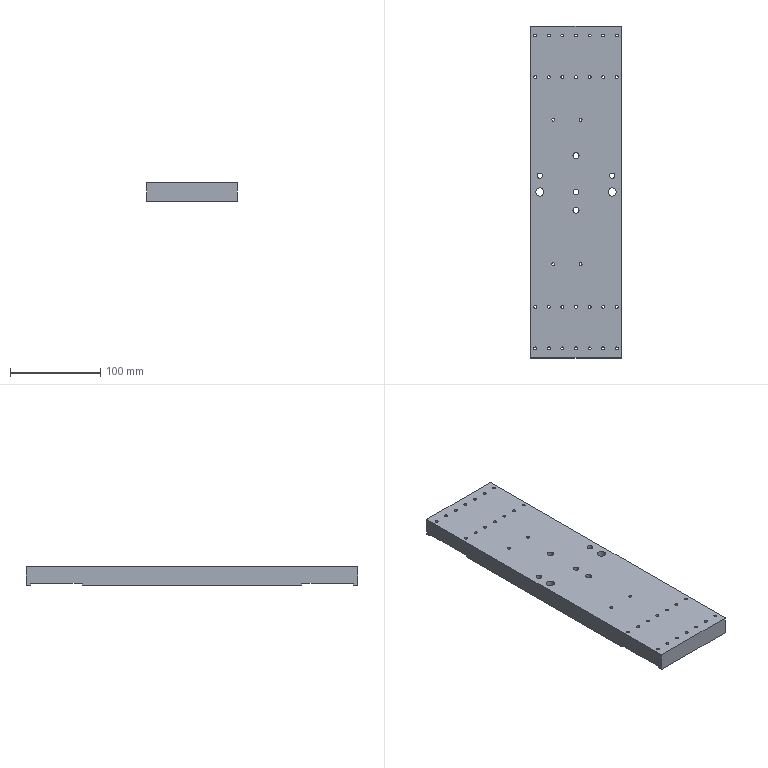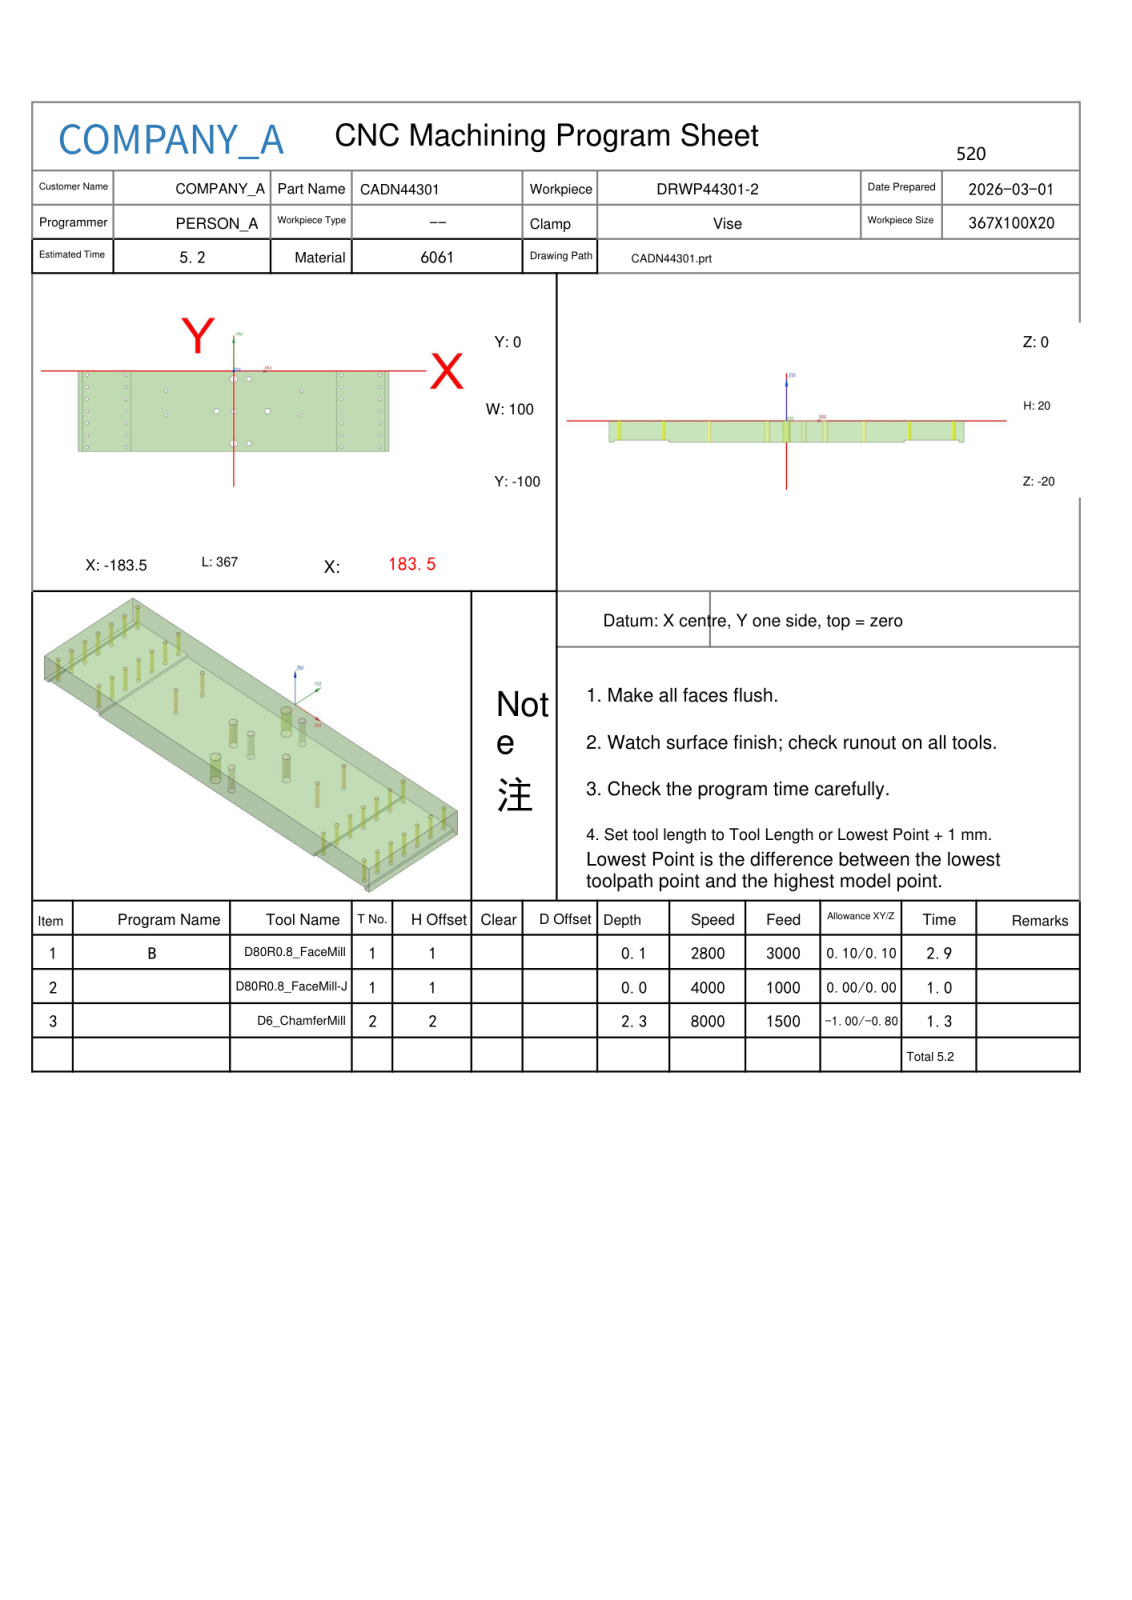NC program | NX | posted by the shop | part box 100 x 367 x 20 mm
Whole program:
%
O0001
(Machine time: 5.71 MIN)
(===Total Tool:2===)
(T1=D80R0.8 FaceMill D=80.  R=0.8  D-  H01 Z=-0.   )
(T2=D6_ChamferMill   D=6.   R=0.   D-  H02 Z=-2.3  )
G80 G90 G17 G49 G40
G91 G28 Z0
M01
N1 T01 M06
(D80R0.8 FaceMill  D=80. R=0.8 H=01 ce=0.10 di=0.10)
G00 G90 G54 X-235.597 Y-23.903 M03 S2800
G43 H01 Z50.
M08
Z6.011
G01 Z4.011 F3000.
X-223.597
X216.397
G02 X223.597 Y-31.103 I0.0 J-7.2
G01 Y-60.737
G02 X215.597 Y-68.737 I-8. J0.0
G01 X-223.597
X-235.597
Z6.011
G00 Y-23.903
Z5.522
G01 Z3.522
X-223.597
X216.397
G02 X223.597 Y-31.103 I0.0 J-7.2
G01 Y-60.737
G02 X215.597 Y-68.737 I-8. J0.0
G01 X-223.597
X-235.597
Z5.522
G00 Y-23.903
Z5.033
G01 Z3.033
X-223.597
X216.397
G02 X223.597 Y-31.103 I0.0 J-7.2
G01 Y-60.737
G02 X215.597 Y-68.737 I-8. J0.0
G01 X-223.597
X-235.597
Z5.033
G00 Y-23.903
Z4.544
G01 Z2.544
X-223.597
X216.397
G02 X223.597 Y-31.103 I0.0 J-7.2
G01 Y-60.737
G02 X215.597 Y-68.737 I-8. J0.0
G01 X-223.597
X-235.597
Z4.544
G00 Y-23.903
Z4.056
G01 Z2.056
X-223.597
X216.397
G02 X223.597 Y-31.103 I0.0 J-7.2
G01 Y-60.737
G02 X215.597 Y-68.737 I-8. J0.0
G01 X-223.597
X-235.597
Z4.056
G00 Y-23.903
Z3.567
G01 Z1.567
X-223.597
X216.397
G02 X223.597 Y-31.103 I0.0 J-7.2
G01 Y-60.737
G02 X215.597 Y-68.737 I-8. J0.0
G01 X-223.597
X-235.597
Z3.567
G00 Y-23.903
Z3.078
G01 Z1.078
X-223.597
X216.397
G02 X223.597 Y-31.103 I0.0 J-7.2
G01 Y-60.737
G02 X215.597 Y-68.737 I-8. J0.0
G01 X-223.597
X-235.597
Z3.078
G00 Y-23.903
Z2.589
G01 Z.589
X-223.597
X216.397
G02 X223.597 Y-31.103 I0.0 J-7.2
G01 Y-60.737
G02 X215.597 Y-68.737 I-8. J0.0
G01 X-223.597
X-235.597
Z2.589
G00 Y-23.903
Z2.1
G01 Z.1
X-223.597
X216.397
G02 X223.597 Y-31.103 I0.0 J-7.2
G01 Y-60.737
G02 X215.597 Y-68.737 I-8. J0.0
G01 X-223.597
X-235.597
Z2.1
G00 Z50.
G91 G28 Z0.0
M05
M09
G91 G28 Z0.0
M01
N2 T01 M06
(D80R0.8 FaceMill-J  D=80. R=0.8 H=01 ce=0.00 di=0.00)
G00 G90 G54 X-235.499 Y-24.001 M03 S4000
G43 H01 Z50.
M08
Z2.
G01 Z0.0 F1000.
X-223.499
X216.299
G02 X223.499 Y-31.201 I0.0 J-7.2
G01 Y-60.639
G02 X215.499 Y-68.639 I-8. J0.0
G01 X-223.499
X-235.499
Z2.
G00 Z50.
G91 G28 Z0.0
M05
M09
G91 G28 Z0.0
M01
N3 T02 M06
(D6_ChamferMill  D=6. R=0. H=02 ce=0.00 di=0.00)
G00 G90 G54 X-173. Y-95. M03 S8000
G43 H02 Z50.
M08
G98 G81 X-173. Y-95. Z-2.2 R3. F1000.
Y-80.
Y-65.
Y-50.
Y-35.
Y-20.
Y-5.
X-127.
Y-20.
Y-35.
Y-50.
Y-65.
Y-80.
Y-95.
X-80. Y-55.
Y-25.
X80. Y-55.
Y-25.
X127. Y-5.
Y-20.
Y-35.
Y-50.
Y-65.
Y-80.
Y-95.
X173.
Y-80.
Y-65.
Y-50.
Y-35.
Y-20.
Y-5.
G80
G00 Z50.
G00 G90 X17.13 Y-10.232 M03 S8000
Z50.
Z-.9
G01 Z-1.4 F600.
X16.5 Y-10.4
G03 X18. Y-11.9 I1.5 J0.0
X19.9 Y-10. I0.0 J1.9
X18. Y-8.1 I-1.9 J0.0
X16.1 Y-10. I0.0 J-1.9
X18. Y-11.9 I1.9 J0.0
X19.5 Y-10.4 I0.0 J1.5
G01 X18.87 Y-10.232
Z-.9
G00 Z50.
X-.87 Y-50.232
Z-.9
G01 Z-1.4
X-1.5 Y-50.4
G03 X0.0 Y-51.9 I1.5 J0.0
X1.9 Y-50. I0.0 J1.9
X0.0 Y-48.1 I-1.9 J0.0
X-1.9 Y-50. I0.0 J-1.9
X0.0 Y-51.9 I1.9 J0.0
X1.5 Y-50.4 I0.0 J1.5
G01 X.87 Y-50.232
Z-.9
G00 Z50.
X17.13 Y-90.232
Z-.9
G01 Z-1.4
X16.5 Y-90.4
G03 X18. Y-91.9 I1.5 J0.0
X19.9 Y-90. I0.0 J1.9
X18. Y-88.1 I-1.9 J0.0
X16.1 Y-90. I0.0 J-1.9
X18. Y-91.9 I1.9 J0.0
X19.5 Y-90.4 I0.0 J1.5
G01 X18.87 Y-90.232
Z-.9
G00 Z50.
G00 G90 X-22. Y-50. M03 S8000
Z50.
Z-.9
G01 Z-1.4 F600.
X-23.
G03 X-20. Y-53. I3. J0.0
X-17. Y-50. I0.0 J3.
X-20. Y-47. I-3. J0.0
X-23. Y-50. I0.0 J-3.
X-20. Y-53. I3. J0.0
X-17. Y-50. I0.0 J3.
G01 X-18.
Z-.9
G00 Z50.
X38.
Z-.9
G01 Z-1.4
X37.
G03 X40. Y-53. I3. J0.0
X43. Y-50. I0.0 J3.
X40. Y-47. I-3. J0.0
X37. Y-50. I0.0 J-3.
X40. Y-53. I3. J0.0
X43. Y-50. I0.0 J3.
G01 X42.
Z-.9
G00 Z50.
G00 G90 X1.5 Y-10. M03 S8000
Z50.
Z-1.8
G01 Z-2.3 F1200.
Y-9.
G03 X0.0 Y-7.5 I-1.5 J0.0
X-2.5 Y-10. I0.0 J-2.5
X0.0 Y-12.5 I2.5 J0.0
X2.5 Y-10. I0.0 J2.5
X0.0 Y-7.5 I-2.5 J0.0
X-1.5 Y-9. I0.0 J-1.5
G01 Y-9.999
Z-1.8
G00 Z50.
X1.5 Y-90.
Z-1.8
G01 Z-2.3
Y-89.
G03 X0.0 Y-87.5 I-1.5 J0.0
X-2.5 Y-90. I0.0 J-2.5
X0.0 Y-92.5 I2.5 J0.0
X2.5 Y-90. I0.0 J2.5
X0.0 Y-87.5 I-2.5 J0.0
X-1.5 Y-89. I0.0 J-1.5
G01 Y-90.
Z-1.8
G00 Z50.
G00 G90 X175.157 Y.7 M03 S7000
Z50.
Z2.5
G01 X183.2 Z-.428 F1500.
X183.278 Z-.456
X183.477 Y.664 Z-.529
X183.665 Y.589 Z-.603
X183.834 Y.477 Z-.677
X183.977 Y.334 Z-.751
X184.089 Y.165 Z-.824
X184.164 Y-.023 Z-.898
X184.2 Y-.222 Z-.972
Y-.3 Z-1.
Y-99.7
G02 X183.2 Y-100.7 I-1. J0.0
G01 X-183.2
G02 X-184.2 Y-99.7 I0.0 J1.
G01 Y-.3
G02 X-183.2 Y.7 I1. J0.0
G01 X183.2
G02 X184.2 Y-.3 I0.0 J-1.
G01 Y-.8
Z1.5
G00 Z50.
M05
M09
G91 G28 Z0.0
G91 G28 Y0.0
M30
%